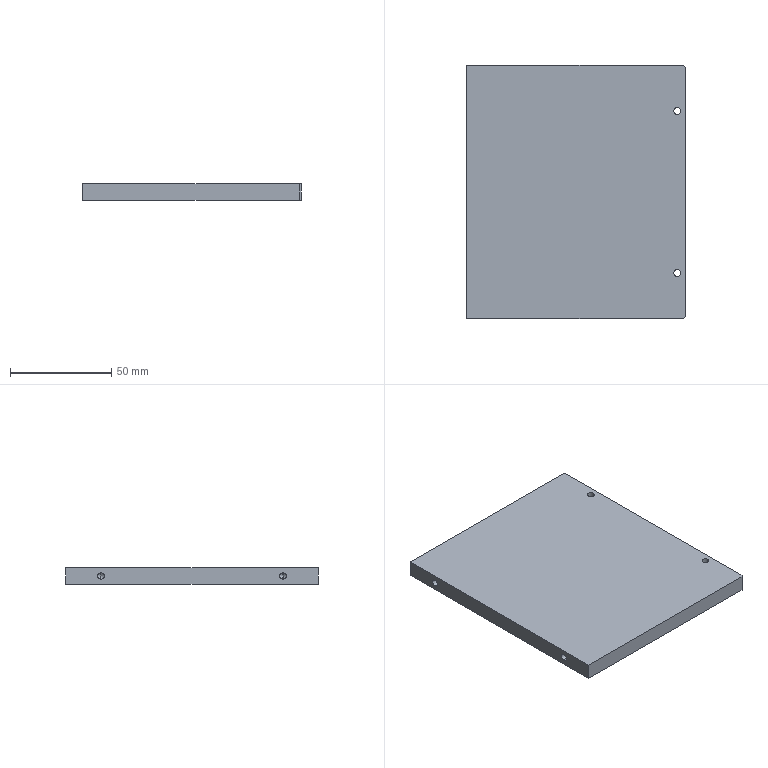Part | STEP file | XL-008 | 1 solid | 26 faces | box 108 x 125 x 8 mm | volume 107538 mm3 | cylinder 12 | plane 10 | cone 4 | commonest cylinder face diameters 3.3 x4 3.4 x4 6 x4
STEP:
#1=CARTESIAN_POINT('',(53.,40.,3.4));
#2=VERTEX_POINT('',#1);
#3=CARTESIAN_POINT('',(47.,40.,3.4));
#4=VERTEX_POINT('',#3);
#5=CARTESIAN_POINT('',(50.,40.,3.4));
#6=DIRECTION('',(0.,0.,-1.));
#7=DIRECTION('',(-1.,0.,0.));
#8=AXIS2_PLACEMENT_3D('',#5,#6,#7);
#9=CIRCLE('',#8,3.);
#10=EDGE_CURVE('',#2,#4,#9,.T.);
#11=ORIENTED_EDGE('',*,*,#10,.F.);
#12=CARTESIAN_POINT('',(53.,40.,0.));
#13=VERTEX_POINT('',#12);
#14=CARTESIAN_POINT('',(53.,40.,0.));
#15=DIRECTION('',(0.,0.,-1.));
#16=VECTOR('',#15,1000.);
#17=LINE('',#14,#16);
#18=EDGE_CURVE('',#2,#13,#17,.T.);
#19=ORIENTED_EDGE('',*,*,#18,.T.);
#20=CARTESIAN_POINT('',(47.,40.,0.));
#21=VERTEX_POINT('',#20);
#22=CARTESIAN_POINT('',(50.,40.,0.));
#23=DIRECTION('',(0.,0.,-1.));
#24=DIRECTION('',(-1.,0.,0.));
#25=AXIS2_PLACEMENT_3D('',#22,#23,#24);
#26=CIRCLE('',#25,3.);
#27=EDGE_CURVE('',#13,#21,#26,.T.);
#28=ORIENTED_EDGE('',*,*,#27,.T.);
#29=CARTESIAN_POINT('',(47.,40.,0.));
#30=DIRECTION('',(0.,0.,-1.));
#31=VECTOR('',#30,1000.);
#32=LINE('',#29,#31);
#33=EDGE_CURVE('',#4,#21,#32,.T.);
#34=ORIENTED_EDGE('',*,*,#33,.F.);
#35=EDGE_LOOP('',(#11,#19,#28,#34));
#36=FACE_OUTER_BOUND('',#35,.T.);
#37=CARTESIAN_POINT('',(50.,40.,0.));
#38=DIRECTION('',(0.,0.,-1.));
#39=DIRECTION('',(-1.,0.,0.));
#40=AXIS2_PLACEMENT_3D('',#37,#38,#39);
#41=CYLINDRICAL_SURFACE('',#40,3.);
#42=ADVANCED_FACE('',(#36),#41,.F.);
#43=CARTESIAN_POINT('',(51.7,40.,8.));
#44=VERTEX_POINT('',#43);
#45=CARTESIAN_POINT('',(48.3,40.,8.));
#46=VERTEX_POINT('',#45);
#47=CARTESIAN_POINT('',(50.,40.,8.));
#48=DIRECTION('',(0.,0.,-1.));
#49=DIRECTION('',(-1.,0.,0.));
#50=AXIS2_PLACEMENT_3D('',#47,#48,#49);
#51=CIRCLE('',#50,1.7);
#52=EDGE_CURVE('',#44,#46,#51,.T.);
#53=ORIENTED_EDGE('',*,*,#52,.F.);
#54=CARTESIAN_POINT('',(51.7,40.,3.4));
#55=VERTEX_POINT('',#54);
#56=CARTESIAN_POINT('',(51.7,40.,0.));
#57=DIRECTION('',(0.,0.,-1.));
#58=VECTOR('',#57,1000.);
#59=LINE('',#56,#58);
#60=EDGE_CURVE('',#44,#55,#59,.T.);
#61=ORIENTED_EDGE('',*,*,#60,.T.);
#62=CARTESIAN_POINT('',(48.3,40.,3.4));
#63=VERTEX_POINT('',#62);
#64=CARTESIAN_POINT('',(50.,40.,3.4));
#65=DIRECTION('',(0.,0.,-1.));
#66=DIRECTION('',(-1.,0.,0.));
#67=AXIS2_PLACEMENT_3D('',#64,#65,#66);
#68=CIRCLE('',#67,1.7);
#69=EDGE_CURVE('',#55,#63,#68,.T.);
#70=ORIENTED_EDGE('',*,*,#69,.T.);
#71=CARTESIAN_POINT('',(48.3,40.,0.));
#72=DIRECTION('',(0.,0.,-1.));
#73=VECTOR('',#72,1000.);
#74=LINE('',#71,#73);
#75=EDGE_CURVE('',#46,#63,#74,.T.);
#76=ORIENTED_EDGE('',*,*,#75,.F.);
#77=EDGE_LOOP('',(#53,#61,#70,#76));
#78=FACE_OUTER_BOUND('',#77,.T.);
#79=CARTESIAN_POINT('',(50.,40.,0.));
#80=DIRECTION('',(0.,0.,-1.));
#81=DIRECTION('',(-1.,0.,0.));
#82=AXIS2_PLACEMENT_3D('',#79,#80,#81);
#83=CYLINDRICAL_SURFACE('',#82,1.7);
#84=ADVANCED_FACE('',(#78),#83,.F.);
#85=CARTESIAN_POINT('',(53.,-40.,3.4));
#86=VERTEX_POINT('',#85);
#87=CARTESIAN_POINT('',(47.,-40.,3.4));
#88=VERTEX_POINT('',#87);
#89=CARTESIAN_POINT('',(50.,-40.,3.4));
#90=DIRECTION('',(0.,0.,-1.));
#91=DIRECTION('',(-1.,0.,0.));
#92=AXIS2_PLACEMENT_3D('',#89,#90,#91);
#93=CIRCLE('',#92,3.);
#94=EDGE_CURVE('',#86,#88,#93,.T.);
#95=ORIENTED_EDGE('',*,*,#94,.F.);
#96=CARTESIAN_POINT('',(53.,-40.,0.));
#97=VERTEX_POINT('',#96);
#98=CARTESIAN_POINT('',(53.,-40.,0.));
#99=DIRECTION('',(0.,0.,-1.));
#100=VECTOR('',#99,1000.);
#101=LINE('',#98,#100);
#102=EDGE_CURVE('',#86,#97,#101,.T.);
#103=ORIENTED_EDGE('',*,*,#102,.T.);
#104=CARTESIAN_POINT('',(47.,-40.,0.));
#105=VERTEX_POINT('',#104);
#106=CARTESIAN_POINT('',(50.,-40.,0.));
#107=DIRECTION('',(0.,0.,-1.));
#108=DIRECTION('',(-1.,0.,0.));
#109=AXIS2_PLACEMENT_3D('',#106,#107,#108);
#110=CIRCLE('',#109,3.);
#111=EDGE_CURVE('',#97,#105,#110,.T.);
#112=ORIENTED_EDGE('',*,*,#111,.T.);
#113=CARTESIAN_POINT('',(47.,-40.,0.));
#114=DIRECTION('',(0.,0.,-1.));
#115=VECTOR('',#114,1000.);
#116=LINE('',#113,#115);
#117=EDGE_CURVE('',#88,#105,#116,.T.);
#118=ORIENTED_EDGE('',*,*,#117,.F.);
#119=EDGE_LOOP('',(#95,#103,#112,#118));
#120=FACE_OUTER_BOUND('',#119,.T.);
#121=CARTESIAN_POINT('',(50.,-40.,0.));
#122=DIRECTION('',(0.,0.,-1.));
#123=DIRECTION('',(-1.,0.,0.));
#124=AXIS2_PLACEMENT_3D('',#121,#122,#123);
#125=CYLINDRICAL_SURFACE('',#124,3.);
#126=ADVANCED_FACE('',(#120),#125,.F.);
#127=CARTESIAN_POINT('',(51.7,-40.,8.));
#128=VERTEX_POINT('',#127);
#129=CARTESIAN_POINT('',(48.3,-40.,8.));
#130=VERTEX_POINT('',#129);
#131=CARTESIAN_POINT('',(50.,-40.,8.));
#132=DIRECTION('',(0.,0.,-1.));
#133=DIRECTION('',(-1.,0.,0.));
#134=AXIS2_PLACEMENT_3D('',#131,#132,#133);
#135=CIRCLE('',#134,1.7);
#136=EDGE_CURVE('',#128,#130,#135,.T.);
#137=ORIENTED_EDGE('',*,*,#136,.F.);
#138=CARTESIAN_POINT('',(51.7,-40.,3.4));
#139=VERTEX_POINT('',#138);
#140=CARTESIAN_POINT('',(51.7,-40.,0.));
#141=DIRECTION('',(0.,0.,-1.));
#142=VECTOR('',#141,1000.);
#143=LINE('',#140,#142);
#144=EDGE_CURVE('',#128,#139,#143,.T.);
#145=ORIENTED_EDGE('',*,*,#144,.T.);
#146=CARTESIAN_POINT('',(48.3,-40.,3.4));
#147=VERTEX_POINT('',#146);
#148=CARTESIAN_POINT('',(50.,-40.,3.4));
#149=DIRECTION('',(0.,0.,-1.));
#150=DIRECTION('',(-1.,0.,0.));
#151=AXIS2_PLACEMENT_3D('',#148,#149,#150);
#152=CIRCLE('',#151,1.7);
#153=EDGE_CURVE('',#139,#147,#152,.T.);
#154=ORIENTED_EDGE('',*,*,#153,.T.);
#155=CARTESIAN_POINT('',(48.3,-40.,0.));
#156=DIRECTION('',(0.,0.,-1.));
#157=VECTOR('',#156,1000.);
#158=LINE('',#155,#157);
#159=EDGE_CURVE('',#130,#147,#158,.T.);
#160=ORIENTED_EDGE('',*,*,#159,.F.);
#161=EDGE_LOOP('',(#137,#145,#154,#160));
#162=FACE_OUTER_BOUND('',#161,.T.);
#163=CARTESIAN_POINT('',(50.,-40.,0.));
#164=DIRECTION('',(0.,0.,-1.));
#165=DIRECTION('',(-1.,0.,0.));
#166=AXIS2_PLACEMENT_3D('',#163,#164,#165);
#167=CYLINDRICAL_SURFACE('',#166,1.7);
#168=ADVANCED_FACE('',(#162),#167,.F.);
#169=CARTESIAN_POINT('',(-43.9,45.,2.35));
#170=VERTEX_POINT('',#169);
#171=CARTESIAN_POINT('',(-43.9,45.,5.65));
#172=VERTEX_POINT('',#171);
#173=CARTESIAN_POINT('',(-43.9,45.,4.));
#174=DIRECTION('',(-1.,0.,0.));
#175=DIRECTION('',(0.,0.,1.));
#176=AXIS2_PLACEMENT_3D('',#173,#174,#175);
#177=CIRCLE('',#176,1.65);
#178=EDGE_CURVE('',#170,#172,#177,.T.);
#179=ORIENTED_EDGE('',*,*,#178,.F.);
#180=CARTESIAN_POINT('',(-54.,45.,2.35));
#181=VERTEX_POINT('',#180);
#182=CARTESIAN_POINT('',(-54.,45.,2.35));
#183=DIRECTION('',(-1.,0.,0.));
#184=VECTOR('',#183,1000.);
#185=LINE('',#182,#184);
#186=EDGE_CURVE('',#170,#181,#185,.T.);
#187=ORIENTED_EDGE('',*,*,#186,.T.);
#188=CARTESIAN_POINT('',(-54.,45.,5.65));
#189=VERTEX_POINT('',#188);
#190=CARTESIAN_POINT('',(-54.,45.,4.));
#191=DIRECTION('',(-1.,0.,0.));
#192=DIRECTION('',(0.,0.,1.));
#193=AXIS2_PLACEMENT_3D('',#190,#191,#192);
#194=CIRCLE('',#193,1.65);
#195=EDGE_CURVE('',#181,#189,#194,.T.);
#196=ORIENTED_EDGE('',*,*,#195,.T.);
#197=CARTESIAN_POINT('',(-54.,45.,5.65));
#198=DIRECTION('',(-1.,0.,0.));
#199=VECTOR('',#198,1000.);
#200=LINE('',#197,#199);
#201=EDGE_CURVE('',#172,#189,#200,.T.);
#202=ORIENTED_EDGE('',*,*,#201,.F.);
#203=EDGE_LOOP('',(#179,#187,#196,#202));
#204=FACE_OUTER_BOUND('',#203,.T.);
#205=CARTESIAN_POINT('',(-54.,45.,4.));
#206=DIRECTION('',(-1.,0.,0.));
#207=DIRECTION('',(0.,0.,1.));
#208=AXIS2_PLACEMENT_3D('',#205,#206,#207);
#209=CYLINDRICAL_SURFACE('',#208,1.65);
#210=ADVANCED_FACE('',(#204),#209,.F.);
#211=CARTESIAN_POINT('',(-42.909,45.,4.));
#212=VERTEX_POINT('',#211);
#213=CARTESIAN_POINT('',(-43.9,45.,5.65));
#214=DIRECTION('',(-0.515,0.,0.8572));
#215=VECTOR('',#214,1000.);
#216=LINE('',#213,#215);
#217=EDGE_CURVE('',#212,#172,#216,.T.);
#218=ORIENTED_EDGE('',*,*,#217,.F.);
#219=CARTESIAN_POINT('',(-43.9,45.,2.35));
#220=DIRECTION('',(-0.515,0.,-0.8572));
#221=VECTOR('',#220,1000.);
#222=LINE('',#219,#221);
#223=EDGE_CURVE('',#212,#170,#222,.T.);
#224=ORIENTED_EDGE('',*,*,#223,.T.);
#225=ORIENTED_EDGE('',*,*,#178,.T.);
#226=EDGE_LOOP('',(#218,#224,#225));
#227=FACE_OUTER_BOUND('',#226,.T.);
#228=CARTESIAN_POINT('',(-43.9,45.,4.));
#229=DIRECTION('',(-1.,0.,0.));
#230=DIRECTION('',(0.,0.,1.));
#231=AXIS2_PLACEMENT_3D('',#228,#229,#230);
#232=CONICAL_SURFACE('',#231,1.65,1.03);
#233=ADVANCED_FACE('',(#227),#232,.F.);
#234=CARTESIAN_POINT('',(-43.9,-45.,2.35));
#235=VERTEX_POINT('',#234);
#236=CARTESIAN_POINT('',(-43.9,-45.,5.65));
#237=VERTEX_POINT('',#236);
#238=CARTESIAN_POINT('',(-43.9,-45.,4.));
#239=DIRECTION('',(-1.,0.,0.));
#240=DIRECTION('',(0.,0.,1.));
#241=AXIS2_PLACEMENT_3D('',#238,#239,#240);
#242=CIRCLE('',#241,1.65);
#243=EDGE_CURVE('',#235,#237,#242,.T.);
#244=ORIENTED_EDGE('',*,*,#243,.F.);
#245=CARTESIAN_POINT('',(-54.,-45.,2.35));
#246=VERTEX_POINT('',#245);
#247=CARTESIAN_POINT('',(-54.,-45.,2.35));
#248=DIRECTION('',(-1.,0.,0.));
#249=VECTOR('',#248,1000.);
#250=LINE('',#247,#249);
#251=EDGE_CURVE('',#235,#246,#250,.T.);
#252=ORIENTED_EDGE('',*,*,#251,.T.);
#253=CARTESIAN_POINT('',(-54.,-45.,5.65));
#254=VERTEX_POINT('',#253);
#255=CARTESIAN_POINT('',(-54.,-45.,4.));
#256=DIRECTION('',(-1.,0.,0.));
#257=DIRECTION('',(0.,0.,1.));
#258=AXIS2_PLACEMENT_3D('',#255,#256,#257);
#259=CIRCLE('',#258,1.65);
#260=EDGE_CURVE('',#246,#254,#259,.T.);
#261=ORIENTED_EDGE('',*,*,#260,.T.);
#262=CARTESIAN_POINT('',(-54.,-45.,5.65));
#263=DIRECTION('',(-1.,0.,0.));
#264=VECTOR('',#263,1000.);
#265=LINE('',#262,#264);
#266=EDGE_CURVE('',#237,#254,#265,.T.);
#267=ORIENTED_EDGE('',*,*,#266,.F.);
#268=EDGE_LOOP('',(#244,#252,#261,#267));
#269=FACE_OUTER_BOUND('',#268,.T.);
#270=CARTESIAN_POINT('',(-54.,-45.,4.));
#271=DIRECTION('',(-1.,0.,0.));
#272=DIRECTION('',(0.,0.,1.));
#273=AXIS2_PLACEMENT_3D('',#270,#271,#272);
#274=CYLINDRICAL_SURFACE('',#273,1.65);
#275=ADVANCED_FACE('',(#269),#274,.F.);
#276=CARTESIAN_POINT('',(-42.909,-45.,4.));
#277=VERTEX_POINT('',#276);
#278=CARTESIAN_POINT('',(-43.9,-45.,5.65));
#279=DIRECTION('',(-0.515,0.,0.8572));
#280=VECTOR('',#279,1000.);
#281=LINE('',#278,#280);
#282=EDGE_CURVE('',#277,#237,#281,.T.);
#283=ORIENTED_EDGE('',*,*,#282,.F.);
#284=CARTESIAN_POINT('',(-43.9,-45.,2.35));
#285=DIRECTION('',(-0.515,0.,-0.8572));
#286=VECTOR('',#285,1000.);
#287=LINE('',#284,#286);
#288=EDGE_CURVE('',#277,#235,#287,.T.);
#289=ORIENTED_EDGE('',*,*,#288,.T.);
#290=ORIENTED_EDGE('',*,*,#243,.T.);
#291=EDGE_LOOP('',(#283,#289,#290));
#292=FACE_OUTER_BOUND('',#291,.T.);
#293=CARTESIAN_POINT('',(-43.9,-45.,4.));
#294=DIRECTION('',(-1.,0.,0.));
#295=DIRECTION('',(0.,0.,1.));
#296=AXIS2_PLACEMENT_3D('',#293,#294,#295);
#297=CONICAL_SURFACE('',#296,1.65,1.03);
#298=ADVANCED_FACE('',(#292),#297,.F.);
#299=CARTESIAN_POINT('',(54.,-61.5,0.));
#300=VERTEX_POINT('',#299);
#301=CARTESIAN_POINT('',(54.,61.5,0.));
#302=VERTEX_POINT('',#301);
#303=CARTESIAN_POINT('',(54.,62.5,0.));
#304=DIRECTION('',(0.,1.,0.));
#305=VECTOR('',#304,1000.);
#306=LINE('',#303,#305);
#307=EDGE_CURVE('',#300,#302,#306,.T.);
#308=ORIENTED_EDGE('',*,*,#307,.T.);
#309=CARTESIAN_POINT('',(54.,61.5,8.));
#310=VERTEX_POINT('',#309);
#311=CARTESIAN_POINT('',(54.,61.5,8.));
#312=DIRECTION('',(0.,0.,1.));
#313=VECTOR('',#312,1000.);
#314=LINE('',#311,#313);
#315=EDGE_CURVE('',#302,#310,#314,.T.);
#316=ORIENTED_EDGE('',*,*,#315,.T.);
#317=CARTESIAN_POINT('',(54.,-61.5,8.));
#318=VERTEX_POINT('',#317);
#319=CARTESIAN_POINT('',(54.,62.5,8.));
#320=DIRECTION('',(0.,1.,0.));
#321=VECTOR('',#320,1000.);
#322=LINE('',#319,#321);
#323=EDGE_CURVE('',#318,#310,#322,.T.);
#324=ORIENTED_EDGE('',*,*,#323,.F.);
#325=CARTESIAN_POINT('',(54.,-61.5,8.));
#326=DIRECTION('',(0.,0.,-1.));
#327=VECTOR('',#326,1000.);
#328=LINE('',#325,#327);
#329=EDGE_CURVE('',#318,#300,#328,.T.);
#330=ORIENTED_EDGE('',*,*,#329,.T.);
#331=EDGE_LOOP('',(#308,#316,#324,#330));
#332=FACE_OUTER_BOUND('',#331,.T.);
#333=CARTESIAN_POINT('',(54.,62.5,8.));
#334=DIRECTION('',(-1.,0.,0.));
#335=DIRECTION('',(0.,-1.,0.));
#336=AXIS2_PLACEMENT_3D('',#333,#334,#335);
#337=PLANE('',#336);
#338=ADVANCED_FACE('',(#332),#337,.F.);
#339=CARTESIAN_POINT('',(53.,62.5,8.));
#340=VERTEX_POINT('',#339);
#341=CARTESIAN_POINT('',(-54.,62.5,8.));
#342=VERTEX_POINT('',#341);
#343=CARTESIAN_POINT('',(-54.,62.5,8.));
#344=DIRECTION('',(-1.,0.,0.));
#345=VECTOR('',#344,1000.);
#346=LINE('',#343,#345);
#347=EDGE_CURVE('',#340,#342,#346,.T.);
#348=ORIENTED_EDGE('',*,*,#347,.F.);
#349=CARTESIAN_POINT('',(53.,62.5,0.));
#350=VERTEX_POINT('',#349);
#351=CARTESIAN_POINT('',(53.,62.5,8.));
#352=DIRECTION('',(0.,0.,-1.));
#353=VECTOR('',#352,1000.);
#354=LINE('',#351,#353);
#355=EDGE_CURVE('',#340,#350,#354,.T.);
#356=ORIENTED_EDGE('',*,*,#355,.T.);
#357=CARTESIAN_POINT('',(-54.,62.5,0.));
#358=VERTEX_POINT('',#357);
#359=CARTESIAN_POINT('',(-54.,62.5,0.));
#360=DIRECTION('',(-1.,0.,0.));
#361=VECTOR('',#360,1000.);
#362=LINE('',#359,#361);
#363=EDGE_CURVE('',#350,#358,#362,.T.);
#364=ORIENTED_EDGE('',*,*,#363,.T.);
#365=CARTESIAN_POINT('',(-54.,62.5,8.));
#366=DIRECTION('',(0.,0.,-1.));
#367=VECTOR('',#366,1000.);
#368=LINE('',#365,#367);
#369=EDGE_CURVE('',#342,#358,#368,.T.);
#370=ORIENTED_EDGE('',*,*,#369,.F.);
#371=EDGE_LOOP('',(#348,#356,#364,#370));
#372=FACE_OUTER_BOUND('',#371,.T.);
#373=CARTESIAN_POINT('',(-54.,62.5,8.));
#374=DIRECTION('',(0.,-1.,0.));
#375=DIRECTION('',(0.,0.,-1.));
#376=AXIS2_PLACEMENT_3D('',#373,#374,#375);
#377=PLANE('',#376);
#378=ADVANCED_FACE('',(#372),#377,.F.);
#379=CARTESIAN_POINT('',(-54.,45.,4.));
#380=DIRECTION('',(-1.,0.,0.));
#381=DIRECTION('',(0.,0.,1.));
#382=AXIS2_PLACEMENT_3D('',#379,#380,#381);
#383=CIRCLE('',#382,1.65);
#384=EDGE_CURVE('',#189,#181,#383,.T.);
#385=ORIENTED_EDGE('',*,*,#384,.F.);
#386=ORIENTED_EDGE('',*,*,#195,.F.);
#387=EDGE_LOOP('',(#385,#386));
#388=FACE_BOUND('',#387,.T.);
#389=CARTESIAN_POINT('',(-54.,-45.,4.));
#390=DIRECTION('',(-1.,0.,0.));
#391=DIRECTION('',(0.,0.,1.));
#392=AXIS2_PLACEMENT_3D('',#389,#390,#391);
#393=CIRCLE('',#392,1.65);
#394=EDGE_CURVE('',#254,#246,#393,.T.);
#395=ORIENTED_EDGE('',*,*,#394,.F.);
#396=ORIENTED_EDGE('',*,*,#260,.F.);
#397=EDGE_LOOP('',(#395,#396));
#398=FACE_BOUND('',#397,.T.);
#399=CARTESIAN_POINT('',(-54.,-62.5,0.));
#400=VERTEX_POINT('',#399);
#401=CARTESIAN_POINT('',(-54.,62.5,0.));
#402=DIRECTION('',(0.,-1.,0.));
#403=VECTOR('',#402,1000.);
#404=LINE('',#401,#403);
#405=EDGE_CURVE('',#358,#400,#404,.T.);
#406=ORIENTED_EDGE('',*,*,#405,.T.);
#407=CARTESIAN_POINT('',(-54.,-62.5,8.));
#408=VERTEX_POINT('',#407);
#409=CARTESIAN_POINT('',(-54.,-62.5,8.));
#410=DIRECTION('',(0.,0.,-1.));
#411=VECTOR('',#410,1000.);
#412=LINE('',#409,#411);
#413=EDGE_CURVE('',#408,#400,#412,.T.);
#414=ORIENTED_EDGE('',*,*,#413,.F.);
#415=CARTESIAN_POINT('',(-54.,62.5,8.));
#416=DIRECTION('',(0.,-1.,0.));
#417=VECTOR('',#416,1000.);
#418=LINE('',#415,#417);
#419=EDGE_CURVE('',#342,#408,#418,.T.);
#420=ORIENTED_EDGE('',*,*,#419,.F.);
#421=ORIENTED_EDGE('',*,*,#369,.T.);
#422=EDGE_LOOP('',(#406,#414,#420,#421));
#423=FACE_OUTER_BOUND('',#422,.T.);
#424=CARTESIAN_POINT('',(-54.,62.5,8.));
#425=DIRECTION('',(1.,0.,0.));
#426=DIRECTION('',(0.,1.,0.));
#427=AXIS2_PLACEMENT_3D('',#424,#425,#426);
#428=PLANE('',#427);
#429=ADVANCED_FACE('',(#388,#398,#423),#428,.F.);
#430=CARTESIAN_POINT('',(53.,-62.5,0.));
#431=VERTEX_POINT('',#430);
#432=CARTESIAN_POINT('',(-54.,-62.5,0.));
#433=DIRECTION('',(1.,0.,0.));
#434=VECTOR('',#433,1000.);
#435=LINE('',#432,#434);
#436=EDGE_CURVE('',#400,#431,#435,.T.);
#437=ORIENTED_EDGE('',*,*,#436,.T.);
#438=CARTESIAN_POINT('',(53.,-62.5,8.));
#439=VERTEX_POINT('',#438);
#440=CARTESIAN_POINT('',(53.,-62.5,8.));
#441=DIRECTION('',(0.,0.,1.));
#442=VECTOR('',#441,1000.);
#443=LINE('',#440,#442);
#444=EDGE_CURVE('',#431,#439,#443,.T.);
#445=ORIENTED_EDGE('',*,*,#444,.T.);
#446=CARTESIAN_POINT('',(-54.,-62.5,8.));
#447=DIRECTION('',(1.,0.,0.));
#448=VECTOR('',#447,1000.);
#449=LINE('',#446,#448);
#450=EDGE_CURVE('',#408,#439,#449,.T.);
#451=ORIENTED_EDGE('',*,*,#450,.F.);
#452=ORIENTED_EDGE('',*,*,#413,.T.);
#453=EDGE_LOOP('',(#437,#445,#451,#452));
#454=FACE_OUTER_BOUND('',#453,.T.);
#455=CARTESIAN_POINT('',(-54.,-62.5,8.));
#456=DIRECTION('',(0.,1.,0.));
#457=DIRECTION('',(0.,0.,1.));
#458=AXIS2_PLACEMENT_3D('',#455,#456,#457);
#459=PLANE('',#458);
#460=ADVANCED_FACE('',(#454),#459,.F.);
#461=CARTESIAN_POINT('',(50.,40.,8.));
#462=DIRECTION('',(0.,0.,-1.));
#463=DIRECTION('',(-1.,0.,0.));
#464=AXIS2_PLACEMENT_3D('',#461,#462,#463);
#465=CIRCLE('',#464,1.7);
#466=EDGE_CURVE('',#46,#44,#465,.T.);
#467=ORIENTED_EDGE('',*,*,#466,.T.);
#468=ORIENTED_EDGE('',*,*,#52,.T.);
#469=EDGE_LOOP('',(#467,#468));
#470=FACE_BOUND('',#469,.T.);
#471=CARTESIAN_POINT('',(50.,-40.,8.));
#472=DIRECTION('',(0.,0.,-1.));
#473=DIRECTION('',(-1.,0.,0.));
#474=AXIS2_PLACEMENT_3D('',#471,#472,#473);
#475=CIRCLE('',#474,1.7);
#476=EDGE_CURVE('',#130,#128,#475,.T.);
#477=ORIENTED_EDGE('',*,*,#476,.T.);
#478=ORIENTED_EDGE('',*,*,#136,.T.);
#479=EDGE_LOOP('',(#477,#478));
#480=FACE_BOUND('',#479,.T.);
#481=ORIENTED_EDGE('',*,*,#323,.T.);
#482=CARTESIAN_POINT('',(57.75,57.75,8.));
#483=DIRECTION('',(-0.7071,0.7071,0.));
#484=VECTOR('',#483,1000.);
#485=LINE('',#482,#484);
#486=EDGE_CURVE('',#310,#340,#485,.T.);
#487=ORIENTED_EDGE('',*,*,#486,.T.);
#488=ORIENTED_EDGE('',*,*,#347,.T.);
#489=ORIENTED_EDGE('',*,*,#419,.T.);
#490=ORIENTED_EDGE('',*,*,#450,.T.);
#491=CARTESIAN_POINT('',(57.75,-57.75,8.));
#492=DIRECTION('',(0.7071,0.7071,0.));
#493=VECTOR('',#492,1000.);
#494=LINE('',#491,#493);
#495=EDGE_CURVE('',#439,#318,#494,.T.);
#496=ORIENTED_EDGE('',*,*,#495,.T.);
#497=EDGE_LOOP('',(#481,#487,#488,#489,#490,#496));
#498=FACE_OUTER_BOUND('',#497,.T.);
#499=CARTESIAN_POINT('',(0.,0.,8.));
#500=DIRECTION('',(0.,0.,1.));
#501=DIRECTION('',(1.,0.,0.));
#502=AXIS2_PLACEMENT_3D('',#499,#500,#501);
#503=PLANE('',#502);
#504=ADVANCED_FACE('',(#470,#480,#498),#503,.T.);
#505=CARTESIAN_POINT('',(50.,40.,0.));
#506=DIRECTION('',(0.,0.,-1.));
#507=DIRECTION('',(-1.,0.,0.));
#508=AXIS2_PLACEMENT_3D('',#505,#506,#507);
#509=CIRCLE('',#508,3.);
#510=EDGE_CURVE('',#21,#13,#509,.T.);
#511=ORIENTED_EDGE('',*,*,#510,.F.);
#512=ORIENTED_EDGE('',*,*,#27,.F.);
#513=EDGE_LOOP('',(#511,#512));
#514=FACE_BOUND('',#513,.T.);
#515=CARTESIAN_POINT('',(50.,-40.,0.));
#516=DIRECTION('',(0.,0.,-1.));
#517=DIRECTION('',(-1.,0.,0.));
#518=AXIS2_PLACEMENT_3D('',#515,#516,#517);
#519=CIRCLE('',#518,3.);
#520=EDGE_CURVE('',#105,#97,#519,.T.);
#521=ORIENTED_EDGE('',*,*,#520,.F.);
#522=ORIENTED_EDGE('',*,*,#111,.F.);
#523=EDGE_LOOP('',(#521,#522));
#524=FACE_BOUND('',#523,.T.);
#525=ORIENTED_EDGE('',*,*,#363,.F.);
#526=CARTESIAN_POINT('',(53.,62.5,0.));
#527=DIRECTION('',(0.7071,-0.7071,0.));
#528=VECTOR('',#527,1000.);
#529=LINE('',#526,#528);
#530=EDGE_CURVE('',#350,#302,#529,.T.);
#531=ORIENTED_EDGE('',*,*,#530,.T.);
#532=ORIENTED_EDGE('',*,*,#307,.F.);
#533=CARTESIAN_POINT('',(54.,-61.5,0.));
#534=DIRECTION('',(-0.7071,-0.7071,0.));
#535=VECTOR('',#534,1000.);
#536=LINE('',#533,#535);
#537=EDGE_CURVE('',#300,#431,#536,.T.);
#538=ORIENTED_EDGE('',*,*,#537,.T.);
#539=ORIENTED_EDGE('',*,*,#436,.F.);
#540=ORIENTED_EDGE('',*,*,#405,.F.);
#541=EDGE_LOOP('',(#525,#531,#532,#538,#539,#540));
#542=FACE_OUTER_BOUND('',#541,.T.);
#543=CARTESIAN_POINT('',(0.,0.,0.));
#544=DIRECTION('',(0.,0.,1.));
#545=DIRECTION('',(1.,0.,0.));
#546=AXIS2_PLACEMENT_3D('',#543,#544,#545);
#547=PLANE('',#546);
#548=ADVANCED_FACE('',(#514,#524,#542),#547,.F.);
#549=ORIENTED_EDGE('',*,*,#288,.F.);
#550=ORIENTED_EDGE('',*,*,#282,.T.);
#551=CARTESIAN_POINT('',(-43.9,-45.,4.));
#552=DIRECTION('',(-1.,0.,0.));
#553=DIRECTION('',(0.,0.,1.));
#554=AXIS2_PLACEMENT_3D('',#551,#552,#553);
#555=CIRCLE('',#554,1.65);
#556=EDGE_CURVE('',#237,#235,#555,.T.);
#557=ORIENTED_EDGE('',*,*,#556,.T.);
#558=EDGE_LOOP('',(#549,#550,#557));
#559=FACE_OUTER_BOUND('',#558,.T.);
#560=CARTESIAN_POINT('',(-43.9,-45.,4.));
#561=DIRECTION('',(-1.,0.,0.));
#562=DIRECTION('',(0.,0.,1.));
#563=AXIS2_PLACEMENT_3D('',#560,#561,#562);
#564=CONICAL_SURFACE('',#563,1.65,1.03);
#565=ADVANCED_FACE('',(#559),#564,.F.);
#566=ORIENTED_EDGE('',*,*,#251,.F.);
#567=ORIENTED_EDGE('',*,*,#556,.F.);
#568=ORIENTED_EDGE('',*,*,#266,.T.);
#569=ORIENTED_EDGE('',*,*,#394,.T.);
#570=EDGE_LOOP('',(#566,#567,#568,#569));
#571=FACE_OUTER_BOUND('',#570,.T.);
#572=CARTESIAN_POINT('',(-54.,-45.,4.));
#573=DIRECTION('',(-1.,0.,0.));
#574=DIRECTION('',(0.,0.,1.));
#575=AXIS2_PLACEMENT_3D('',#572,#573,#574);
#576=CYLINDRICAL_SURFACE('',#575,1.65);
#577=ADVANCED_FACE('',(#571),#576,.F.);
#578=ORIENTED_EDGE('',*,*,#223,.F.);
#579=ORIENTED_EDGE('',*,*,#217,.T.);
#580=CARTESIAN_POINT('',(-43.9,45.,4.));
#581=DIRECTION('',(-1.,0.,0.));
#582=DIRECTION('',(0.,0.,1.));
#583=AXIS2_PLACEMENT_3D('',#580,#581,#582);
#584=CIRCLE('',#583,1.65);
#585=EDGE_CURVE('',#172,#170,#584,.T.);
#586=ORIENTED_EDGE('',*,*,#585,.T.);
#587=EDGE_LOOP('',(#578,#579,#586));
#588=FACE_OUTER_BOUND('',#587,.T.);
#589=CARTESIAN_POINT('',(-43.9,45.,4.));
#590=DIRECTION('',(-1.,0.,0.));
#591=DIRECTION('',(0.,0.,1.));
#592=AXIS2_PLACEMENT_3D('',#589,#590,#591);
#593=CONICAL_SURFACE('',#592,1.65,1.03);
#594=ADVANCED_FACE('',(#588),#593,.F.);
#595=ORIENTED_EDGE('',*,*,#186,.F.);
#596=ORIENTED_EDGE('',*,*,#585,.F.);
#597=ORIENTED_EDGE('',*,*,#201,.T.);
#598=ORIENTED_EDGE('',*,*,#384,.T.);
#599=EDGE_LOOP('',(#595,#596,#597,#598));
#600=FACE_OUTER_BOUND('',#599,.T.);
#601=CARTESIAN_POINT('',(-54.,45.,4.));
#602=DIRECTION('',(-1.,0.,0.));
#603=DIRECTION('',(0.,0.,1.));
#604=AXIS2_PLACEMENT_3D('',#601,#602,#603);
#605=CYLINDRICAL_SURFACE('',#604,1.65);
#606=ADVANCED_FACE('',(#600),#605,.F.);
#607=ORIENTED_EDGE('',*,*,#144,.F.);
#608=ORIENTED_EDGE('',*,*,#476,.F.);
#609=ORIENTED_EDGE('',*,*,#159,.T.);
#610=CARTESIAN_POINT('',(50.,-40.,3.4));
#611=DIRECTION('',(0.,0.,-1.));
#612=DIRECTION('',(-1.,0.,0.));
#613=AXIS2_PLACEMENT_3D('',#610,#611,#612);
#614=CIRCLE('',#613,1.7);
#615=EDGE_CURVE('',#147,#139,#614,.T.);
#616=ORIENTED_EDGE('',*,*,#615,.T.);
#617=EDGE_LOOP('',(#607,#608,#609,#616));
#618=FACE_OUTER_BOUND('',#617,.T.);
#619=CARTESIAN_POINT('',(50.,-40.,0.));
#620=DIRECTION('',(0.,0.,-1.));
#621=DIRECTION('',(-1.,0.,0.));
#622=AXIS2_PLACEMENT_3D('',#619,#620,#621);
#623=CYLINDRICAL_SURFACE('',#622,1.7);
#624=ADVANCED_FACE('',(#618),#623,.F.);
#625=ORIENTED_EDGE('',*,*,#615,.F.);
#626=ORIENTED_EDGE('',*,*,#153,.F.);
#627=EDGE_LOOP('',(#625,#626));
#628=FACE_BOUND('',#627,.T.);
#629=CARTESIAN_POINT('',(50.,-40.,3.4));
#630=DIRECTION('',(0.,0.,-1.));
#631=DIRECTION('',(-1.,0.,0.));
#632=AXIS2_PLACEMENT_3D('',#629,#630,#631);
#633=CIRCLE('',#632,3.);
#634=EDGE_CURVE('',#88,#86,#633,.T.);
#635=ORIENTED_EDGE('',*,*,#634,.T.);
#636=ORIENTED_EDGE('',*,*,#94,.T.);
#637=EDGE_LOOP('',(#635,#636));
#638=FACE_OUTER_BOUND('',#637,.T.);
#639=CARTESIAN_POINT('',(51.7,-40.,3.4));
#640=DIRECTION('',(0.,0.,1.));
#641=DIRECTION('',(1.,0.,0.));
#642=AXIS2_PLACEMENT_3D('',#639,#640,#641);
#643=PLANE('',#642);
#644=ADVANCED_FACE('',(#628,#638),#643,.F.);
#645=ORIENTED_EDGE('',*,*,#102,.F.);
#646=ORIENTED_EDGE('',*,*,#634,.F.);
#647=ORIENTED_EDGE('',*,*,#117,.T.);
#648=ORIENTED_EDGE('',*,*,#520,.T.);
#649=EDGE_LOOP('',(#645,#646,#647,#648));
#650=FACE_OUTER_BOUND('',#649,.T.);
#651=CARTESIAN_POINT('',(50.,-40.,0.));
#652=DIRECTION('',(0.,0.,-1.));
#653=DIRECTION('',(-1.,0.,0.));
#654=AXIS2_PLACEMENT_3D('',#651,#652,#653);
#655=CYLINDRICAL_SURFACE('',#654,3.);
#656=ADVANCED_FACE('',(#650),#655,.F.);
#657=ORIENTED_EDGE('',*,*,#60,.F.);
#658=ORIENTED_EDGE('',*,*,#466,.F.);
#659=ORIENTED_EDGE('',*,*,#75,.T.);
#660=CARTESIAN_POINT('',(50.,40.,3.4));
#661=DIRECTION('',(0.,0.,-1.));
#662=DIRECTION('',(-1.,0.,0.));
#663=AXIS2_PLACEMENT_3D('',#660,#661,#662);
#664=CIRCLE('',#663,1.7);
#665=EDGE_CURVE('',#63,#55,#664,.T.);
#666=ORIENTED_EDGE('',*,*,#665,.T.);
#667=EDGE_LOOP('',(#657,#658,#659,#666));
#668=FACE_OUTER_BOUND('',#667,.T.);
#669=CARTESIAN_POINT('',(50.,40.,0.));
#670=DIRECTION('',(0.,0.,-1.));
#671=DIRECTION('',(-1.,0.,0.));
#672=AXIS2_PLACEMENT_3D('',#669,#670,#671);
#673=CYLINDRICAL_SURFACE('',#672,1.7);
#674=ADVANCED_FACE('',(#668),#673,.F.);
#675=ORIENTED_EDGE('',*,*,#665,.F.);
#676=ORIENTED_EDGE('',*,*,#69,.F.);
#677=EDGE_LOOP('',(#675,#676));
#678=FACE_BOUND('',#677,.T.);
#679=CARTESIAN_POINT('',(50.,40.,3.4));
#680=DIRECTION('',(0.,0.,-1.));
#681=DIRECTION('',(-1.,0.,0.));
#682=AXIS2_PLACEMENT_3D('',#679,#680,#681);
#683=CIRCLE('',#682,3.);
#684=EDGE_CURVE('',#4,#2,#683,.T.);
#685=ORIENTED_EDGE('',*,*,#684,.T.);
#686=ORIENTED_EDGE('',*,*,#10,.T.);
#687=EDGE_LOOP('',(#685,#686));
#688=FACE_OUTER_BOUND('',#687,.T.);
#689=CARTESIAN_POINT('',(51.7,40.,3.4));
#690=DIRECTION('',(0.,0.,1.));
#691=DIRECTION('',(1.,0.,0.));
#692=AXIS2_PLACEMENT_3D('',#689,#690,#691);
#693=PLANE('',#692);
#694=ADVANCED_FACE('',(#678,#688),#693,.F.);
#695=ORIENTED_EDGE('',*,*,#18,.F.);
#696=ORIENTED_EDGE('',*,*,#684,.F.);
#697=ORIENTED_EDGE('',*,*,#33,.T.);
#698=ORIENTED_EDGE('',*,*,#510,.T.);
#699=EDGE_LOOP('',(#695,#696,#697,#698));
#700=FACE_OUTER_BOUND('',#699,.T.);
#701=CARTESIAN_POINT('',(50.,40.,0.));
#702=DIRECTION('',(0.,0.,-1.));
#703=DIRECTION('',(-1.,0.,0.));
#704=AXIS2_PLACEMENT_3D('',#701,#702,#703);
#705=CYLINDRICAL_SURFACE('',#704,3.);
#706=ADVANCED_FACE('',(#700),#705,.F.);
#707=ORIENTED_EDGE('',*,*,#486,.F.);
#708=ORIENTED_EDGE('',*,*,#315,.F.);
#709=ORIENTED_EDGE('',*,*,#530,.F.);
#710=ORIENTED_EDGE('',*,*,#355,.F.);
#711=EDGE_LOOP('',(#707,#708,#709,#710));
#712=FACE_OUTER_BOUND('',#711,.T.);
#713=CARTESIAN_POINT('',(53.,62.5,8.));
#714=DIRECTION('',(-0.7071,-0.7071,0.));
#715=DIRECTION('',(0.,0.,-1.));
#716=AXIS2_PLACEMENT_3D('',#713,#714,#715);
#717=PLANE('',#716);
#718=ADVANCED_FACE('',(#712),#717,.F.);
#719=ORIENTED_EDGE('',*,*,#495,.F.);
#720=ORIENTED_EDGE('',*,*,#444,.F.);
#721=ORIENTED_EDGE('',*,*,#537,.F.);
#722=ORIENTED_EDGE('',*,*,#329,.F.);
#723=EDGE_LOOP('',(#719,#720,#721,#722));
#724=FACE_OUTER_BOUND('',#723,.T.);
#725=CARTESIAN_POINT('',(54.,-61.5,8.));
#726=DIRECTION('',(-0.7071,0.7071,0.));
#727=DIRECTION('',(0.,0.,-1.));
#728=AXIS2_PLACEMENT_3D('',#725,#726,#727);
#729=PLANE('',#728);
#730=ADVANCED_FACE('',(#724),#729,.F.);
#731=CLOSED_SHELL('',(#42,#84,#126,#168,#210,#233,#275,#298,#338,#378,#429,#460,#504,#548,#565,#577,#594,#606,#624,#644,#656,#674,#694,#706,#718,#730));
#732=MANIFOLD_SOLID_BREP('',#731);
#733=CARTESIAN_POINT('',(0.,0.,0.));
#734=DIRECTION('',(0.,0.,1.));
#735=DIRECTION('',(1.,0.,0.));
#736=AXIS2_PLACEMENT_3D('',#733,#734,#735);
#737=(LENGTH_UNIT()NAMED_UNIT(*)SI_UNIT(.MILLI.,.METRE.));
#738=UNCERTAINTY_MEASURE_WITH_UNIT(LENGTH_MEASURE(0.00001),#737,'','');
#739=(NAMED_UNIT(*)PLANE_ANGLE_UNIT()SI_UNIT($,.RADIAN.));
#740=(NAMED_UNIT(*)SI_UNIT($,.STERADIAN.)SOLID_ANGLE_UNIT());
#741=(GEOMETRIC_REPRESENTATION_CONTEXT(3)GLOBAL_UNCERTAINTY_ASSIGNED_CONTEXT((#738))GLOBAL_UNIT_ASSIGNED_CONTEXT((#737,#739,#740))REPRESENTATION_CONTEXT('',''));
#742=ADVANCED_BREP_SHAPE_REPRESENTATION('',(#732,#736),#741);